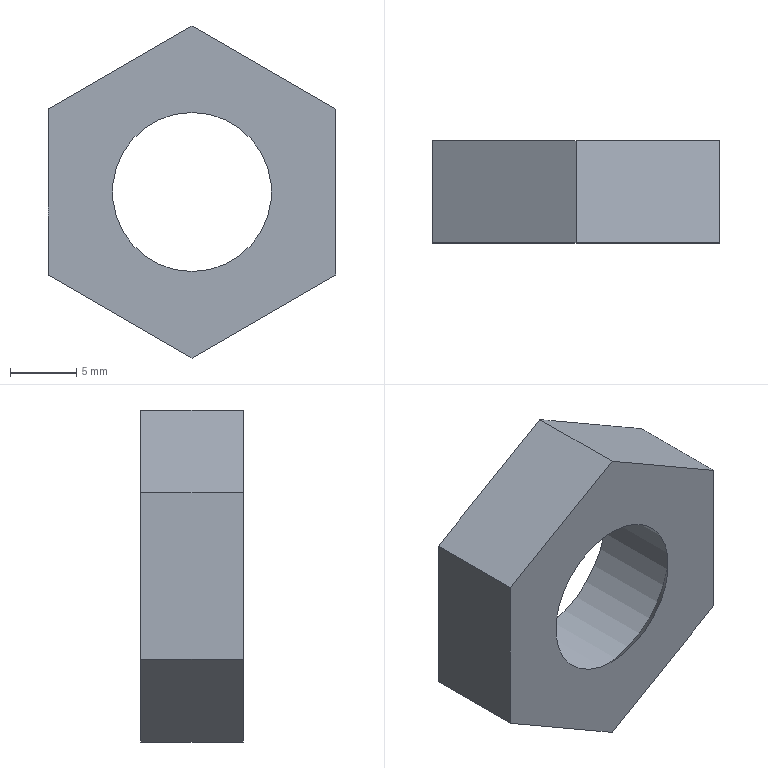Part | NX | features solid 2 | 1 solid | 10 faces | box 21.7 x 7.7 x 25.057 mm | volume 1976 mm3 | plane 8 | cylinder 1 | cone 1 | commonest cylinder face diameters 14 x1
STEP:
#1=CARTESIAN_POINT('',(0.,174.7,-30.529));
#2=VERTEX_POINT('',#1);
#3=CARTESIAN_POINT('',(10.85,174.7,-24.264));
#4=VERTEX_POINT('',#3);
#5=CARTESIAN_POINT('',(0.,174.7,-30.529));
#6=DIRECTION('',(0.866,0.,0.5));
#7=VECTOR('',#6,1000.);
#8=LINE('',#5,#7);
#9=EDGE_CURVE('',#2,#4,#8,.T.);
#10=ORIENTED_EDGE('',*,*,#9,.T.);
#11=CARTESIAN_POINT('',(10.85,167.,-24.264));
#12=VERTEX_POINT('',#11);
#13=CARTESIAN_POINT('',(10.85,167.,-24.264));
#14=DIRECTION('',(0.,1.,0.));
#15=VECTOR('',#14,1000.);
#16=LINE('',#13,#15);
#17=EDGE_CURVE('',#12,#4,#16,.T.);
#18=ORIENTED_EDGE('',*,*,#17,.F.);
#19=CARTESIAN_POINT('',(0.,167.,-30.529));
#20=VERTEX_POINT('',#19);
#21=CARTESIAN_POINT('',(0.,167.,-30.529));
#22=DIRECTION('',(0.866,0.,0.5));
#23=VECTOR('',#22,1000.);
#24=LINE('',#21,#23);
#25=EDGE_CURVE('',#20,#12,#24,.T.);
#26=ORIENTED_EDGE('',*,*,#25,.F.);
#27=CARTESIAN_POINT('',(0.,167.,-30.529));
#28=DIRECTION('',(0.,1.,0.));
#29=VECTOR('',#28,1000.);
#30=LINE('',#27,#29);
#31=EDGE_CURVE('',#20,#2,#30,.T.);
#32=ORIENTED_EDGE('',*,*,#31,.T.);
#33=EDGE_LOOP('',(#10,#18,#26,#32));
#34=FACE_BOUND('',#33,.T.);
#35=CARTESIAN_POINT('',(0.,167.,-30.529));
#36=DIRECTION('',(-0.5,0.,0.866));
#37=DIRECTION('',(0.,1.,0.));
#38=AXIS2_PLACEMENT_3D('',#35,#36,#37);
#39=PLANE('',#38);
#40=ADVANCED_FACE('',(#34),#39,.F.);
#41=CARTESIAN_POINT('',(10.85,174.7,-11.736));
#42=VERTEX_POINT('',#41);
#43=CARTESIAN_POINT('',(10.85,174.7,-24.264));
#44=DIRECTION('',(0.,0.,1.));
#45=VECTOR('',#44,1000.);
#46=LINE('',#43,#45);
#47=EDGE_CURVE('',#4,#42,#46,.T.);
#48=ORIENTED_EDGE('',*,*,#47,.T.);
#49=CARTESIAN_POINT('',(10.85,167.,-11.736));
#50=VERTEX_POINT('',#49);
#51=CARTESIAN_POINT('',(10.85,167.,-11.736));
#52=DIRECTION('',(0.,1.,0.));
#53=VECTOR('',#52,1000.);
#54=LINE('',#51,#53);
#55=EDGE_CURVE('',#50,#42,#54,.T.);
#56=ORIENTED_EDGE('',*,*,#55,.F.);
#57=CARTESIAN_POINT('',(10.85,167.,-24.264));
#58=DIRECTION('',(0.,0.,1.));
#59=VECTOR('',#58,1000.);
#60=LINE('',#57,#59);
#61=EDGE_CURVE('',#12,#50,#60,.T.);
#62=ORIENTED_EDGE('',*,*,#61,.F.);
#63=ORIENTED_EDGE('',*,*,#17,.T.);
#64=EDGE_LOOP('',(#48,#56,#62,#63));
#65=FACE_BOUND('',#64,.T.);
#66=CARTESIAN_POINT('',(10.85,167.,-24.264));
#67=DIRECTION('',(-1.,0.,0.));
#68=DIRECTION('',(0.,0.,-1.));
#69=AXIS2_PLACEMENT_3D('',#66,#67,#68);
#70=PLANE('',#69);
#71=ADVANCED_FACE('',(#65),#70,.F.);
#72=CARTESIAN_POINT('',(0.,174.7,-5.471));
#73=VERTEX_POINT('',#72);
#74=CARTESIAN_POINT('',(10.85,174.7,-11.736));
#75=DIRECTION('',(-0.866,0.,0.5));
#76=VECTOR('',#75,1000.);
#77=LINE('',#74,#76);
#78=EDGE_CURVE('',#42,#73,#77,.T.);
#79=ORIENTED_EDGE('',*,*,#78,.T.);
#80=CARTESIAN_POINT('',(0.,167.,-5.471));
#81=VERTEX_POINT('',#80);
#82=CARTESIAN_POINT('',(0.,167.,-5.471));
#83=DIRECTION('',(0.,1.,0.));
#84=VECTOR('',#83,1000.);
#85=LINE('',#82,#84);
#86=EDGE_CURVE('',#81,#73,#85,.T.);
#87=ORIENTED_EDGE('',*,*,#86,.F.);
#88=CARTESIAN_POINT('',(10.85,167.,-11.736));
#89=DIRECTION('',(-0.866,0.,0.5));
#90=VECTOR('',#89,1000.);
#91=LINE('',#88,#90);
#92=EDGE_CURVE('',#50,#81,#91,.T.);
#93=ORIENTED_EDGE('',*,*,#92,.F.);
#94=ORIENTED_EDGE('',*,*,#55,.T.);
#95=EDGE_LOOP('',(#79,#87,#93,#94));
#96=FACE_BOUND('',#95,.T.);
#97=CARTESIAN_POINT('',(10.85,167.,-11.736));
#98=DIRECTION('',(-0.5,0.,-0.866));
#99=DIRECTION('',(0.866,0.,-0.5));
#100=AXIS2_PLACEMENT_3D('',#97,#98,#99);
#101=PLANE('',#100);
#102=ADVANCED_FACE('',(#96),#101,.F.);
#103=CARTESIAN_POINT('',(-10.85,174.7,-11.736));
#104=VERTEX_POINT('',#103);
#105=CARTESIAN_POINT('',(0.,174.7,-5.471));
#106=DIRECTION('',(-0.866,0.,-0.5));
#107=VECTOR('',#106,1000.);
#108=LINE('',#105,#107);
#109=EDGE_CURVE('',#73,#104,#108,.T.);
#110=ORIENTED_EDGE('',*,*,#109,.T.);
#111=CARTESIAN_POINT('',(-10.85,167.,-11.736));
#112=VERTEX_POINT('',#111);
#113=CARTESIAN_POINT('',(-10.85,167.,-11.736));
#114=DIRECTION('',(0.,1.,0.));
#115=VECTOR('',#114,1000.);
#116=LINE('',#113,#115);
#117=EDGE_CURVE('',#112,#104,#116,.T.);
#118=ORIENTED_EDGE('',*,*,#117,.F.);
#119=CARTESIAN_POINT('',(0.,167.,-5.471));
#120=DIRECTION('',(-0.866,0.,-0.5));
#121=VECTOR('',#120,1000.);
#122=LINE('',#119,#121);
#123=EDGE_CURVE('',#81,#112,#122,.T.);
#124=ORIENTED_EDGE('',*,*,#123,.F.);
#125=ORIENTED_EDGE('',*,*,#86,.T.);
#126=EDGE_LOOP('',(#110,#118,#124,#125));
#127=FACE_BOUND('',#126,.T.);
#128=CARTESIAN_POINT('',(0.,167.,-5.471));
#129=DIRECTION('',(0.5,0.,-0.866));
#130=DIRECTION('',(0.866,0.,0.5));
#131=AXIS2_PLACEMENT_3D('',#128,#129,#130);
#132=PLANE('',#131);
#133=ADVANCED_FACE('',(#127),#132,.F.);
#134=CARTESIAN_POINT('',(-10.85,174.7,-24.264));
#135=VERTEX_POINT('',#134);
#136=CARTESIAN_POINT('',(-10.85,174.7,-11.736));
#137=DIRECTION('',(0.,0.,-1.));
#138=VECTOR('',#137,1000.);
#139=LINE('',#136,#138);
#140=EDGE_CURVE('',#104,#135,#139,.T.);
#141=ORIENTED_EDGE('',*,*,#140,.T.);
#142=CARTESIAN_POINT('',(-10.85,167.,-24.264));
#143=VERTEX_POINT('',#142);
#144=CARTESIAN_POINT('',(-10.85,167.,-24.264));
#145=DIRECTION('',(0.,1.,0.));
#146=VECTOR('',#145,1000.);
#147=LINE('',#144,#146);
#148=EDGE_CURVE('',#143,#135,#147,.T.);
#149=ORIENTED_EDGE('',*,*,#148,.F.);
#150=CARTESIAN_POINT('',(-10.85,167.,-11.736));
#151=DIRECTION('',(0.,0.,-1.));
#152=VECTOR('',#151,1000.);
#153=LINE('',#150,#152);
#154=EDGE_CURVE('',#112,#143,#153,.T.);
#155=ORIENTED_EDGE('',*,*,#154,.F.);
#156=ORIENTED_EDGE('',*,*,#117,.T.);
#157=EDGE_LOOP('',(#141,#149,#155,#156));
#158=FACE_BOUND('',#157,.T.);
#159=CARTESIAN_POINT('',(-10.85,167.,-11.736));
#160=DIRECTION('',(1.,0.,0.));
#161=DIRECTION('',(0.,0.,1.));
#162=AXIS2_PLACEMENT_3D('',#159,#160,#161);
#163=PLANE('',#162);
#164=ADVANCED_FACE('',(#158),#163,.F.);
#165=CARTESIAN_POINT('',(-10.85,174.7,-24.264));
#166=DIRECTION('',(0.866,0.,-0.5));
#167=VECTOR('',#166,1000.);
#168=LINE('',#165,#167);
#169=EDGE_CURVE('',#135,#2,#168,.T.);
#170=ORIENTED_EDGE('',*,*,#169,.T.);
#171=ORIENTED_EDGE('',*,*,#31,.F.);
#172=CARTESIAN_POINT('',(-10.85,167.,-24.264));
#173=DIRECTION('',(0.866,0.,-0.5));
#174=VECTOR('',#173,1000.);
#175=LINE('',#172,#174);
#176=EDGE_CURVE('',#143,#20,#175,.T.);
#177=ORIENTED_EDGE('',*,*,#176,.F.);
#178=ORIENTED_EDGE('',*,*,#148,.T.);
#179=EDGE_LOOP('',(#170,#171,#177,#178));
#180=FACE_BOUND('',#179,.T.);
#181=CARTESIAN_POINT('',(-10.85,167.,-24.264));
#182=DIRECTION('',(0.5,0.,0.866));
#183=DIRECTION('',(-0.866,0.,0.5));
#184=AXIS2_PLACEMENT_3D('',#181,#182,#183);
#185=PLANE('',#184);
#186=ADVANCED_FACE('',(#180),#185,.F.);
#187=CARTESIAN_POINT('',(0.,167.,-12.));
#188=VERTEX_POINT('',#187);
#189=CARTESIAN_POINT('',(0.,167.,-18.));
#190=DIRECTION('',(0.,-1.,0.));
#191=DIRECTION('',(0.,0.,1.));
#192=AXIS2_PLACEMENT_3D('',#189,#190,#191);
#193=CIRCLE('',#192,6.);
#194=EDGE_CURVE('',#188,#188,#193,.T.);
#195=ORIENTED_EDGE('',*,*,#194,.F.);
#196=EDGE_LOOP('',(#195));
#197=FACE_BOUND('',#196,.T.);
#198=ORIENTED_EDGE('',*,*,#25,.T.);
#199=ORIENTED_EDGE('',*,*,#61,.T.);
#200=ORIENTED_EDGE('',*,*,#92,.T.);
#201=ORIENTED_EDGE('',*,*,#123,.T.);
#202=ORIENTED_EDGE('',*,*,#154,.T.);
#203=ORIENTED_EDGE('',*,*,#176,.T.);
#204=EDGE_LOOP('',(#198,#199,#200,#201,#202,#203));
#205=FACE_BOUND('',#204,.T.);
#206=CARTESIAN_POINT('',(123.481,167.,-171.875));
#207=DIRECTION('',(0.,-1.,0.));
#208=DIRECTION('',(-0.866,0.,-0.5));
#209=AXIS2_PLACEMENT_3D('',#206,#207,#208);
#210=PLANE('',#209);
#211=ADVANCED_FACE('',(#197,#205),#210,.T.);
#212=CARTESIAN_POINT('',(0.,174.7,-11.));
#213=VERTEX_POINT('',#212);
#214=CARTESIAN_POINT('',(0.,174.7,-18.));
#215=DIRECTION('',(0.,-1.,0.));
#216=DIRECTION('',(0.,0.,1.));
#217=AXIS2_PLACEMENT_3D('',#214,#215,#216);
#218=CIRCLE('',#217,7.);
#219=EDGE_CURVE('',#213,#213,#218,.T.);
#220=ORIENTED_EDGE('',*,*,#219,.T.);
#221=EDGE_LOOP('',(#220));
#222=FACE_BOUND('',#221,.T.);
#223=ORIENTED_EDGE('',*,*,#9,.F.);
#224=ORIENTED_EDGE('',*,*,#169,.F.);
#225=ORIENTED_EDGE('',*,*,#140,.F.);
#226=ORIENTED_EDGE('',*,*,#109,.F.);
#227=ORIENTED_EDGE('',*,*,#78,.F.);
#228=ORIENTED_EDGE('',*,*,#47,.F.);
#229=EDGE_LOOP('',(#223,#224,#225,#226,#227,#228));
#230=FACE_BOUND('',#229,.T.);
#231=CARTESIAN_POINT('',(123.481,174.7,-171.875));
#232=DIRECTION('',(0.,-1.,0.));
#233=DIRECTION('',(-0.866,0.,-0.5));
#234=AXIS2_PLACEMENT_3D('',#231,#232,#233);
#235=PLANE('',#234);
#236=ADVANCED_FACE('',(#222,#230),#235,.F.);
#237=CARTESIAN_POINT('',(0.,168.,-11.));
#238=VERTEX_POINT('',#237);
#239=CARTESIAN_POINT('',(0.,168.,-18.));
#240=DIRECTION('',(0.,-1.,0.));
#241=DIRECTION('',(0.,0.,1.));
#242=AXIS2_PLACEMENT_3D('',#239,#240,#241);
#243=CIRCLE('',#242,7.);
#244=EDGE_CURVE('',#238,#238,#243,.T.);
#245=ORIENTED_EDGE('',*,*,#244,.T.);
#246=EDGE_LOOP('',(#245));
#247=FACE_BOUND('',#246,.T.);
#248=ORIENTED_EDGE('',*,*,#219,.F.);
#249=EDGE_LOOP('',(#248));
#250=FACE_BOUND('',#249,.T.);
#251=CARTESIAN_POINT('',(0.,195.,-18.));
#252=DIRECTION('',(0.,-1.,0.));
#253=DIRECTION('',(0.,0.,-1.));
#254=AXIS2_PLACEMENT_3D('',#251,#252,#253);
#255=CYLINDRICAL_SURFACE('',#254,7.);
#256=ADVANCED_FACE('',(#247,#250),#255,.F.);
#257=ORIENTED_EDGE('',*,*,#244,.F.);
#258=EDGE_LOOP('',(#257));
#259=FACE_BOUND('',#258,.T.);
#260=ORIENTED_EDGE('',*,*,#194,.T.);
#261=EDGE_LOOP('',(#260));
#262=FACE_BOUND('',#261,.T.);
#263=CARTESIAN_POINT('',(0.,167.,-18.));
#264=DIRECTION('',(0.,1.,0.));
#265=DIRECTION('',(0.,0.,-1.));
#266=AXIS2_PLACEMENT_3D('',#263,#264,#265);
#267=CONICAL_SURFACE('',#266,6.,0.7854);
#268=ADVANCED_FACE('',(#259,#262),#267,.F.);
#269=CLOSED_SHELL('',(#40,#71,#102,#133,#164,#186,#211,#236,#256,#268));
#270=MANIFOLD_SOLID_BREP('',#269);
#271=(LENGTH_UNIT()NAMED_UNIT(*)SI_UNIT(.MILLI.,.METRE.));
#272=UNCERTAINTY_MEASURE_WITH_UNIT(LENGTH_MEASURE(0.00001),#271,'','');
#273=(NAMED_UNIT(*)PLANE_ANGLE_UNIT()SI_UNIT($,.RADIAN.));
#274=(NAMED_UNIT(*)SI_UNIT($,.STERADIAN.)SOLID_ANGLE_UNIT());
#275=(GEOMETRIC_REPRESENTATION_CONTEXT(3)GLOBAL_UNCERTAINTY_ASSIGNED_CONTEXT((#272))GLOBAL_UNIT_ASSIGNED_CONTEXT((#271,#273,#274))REPRESENTATION_CONTEXT('',''));
#276=ADVANCED_BREP_SHAPE_REPRESENTATION('',(#270),#275);